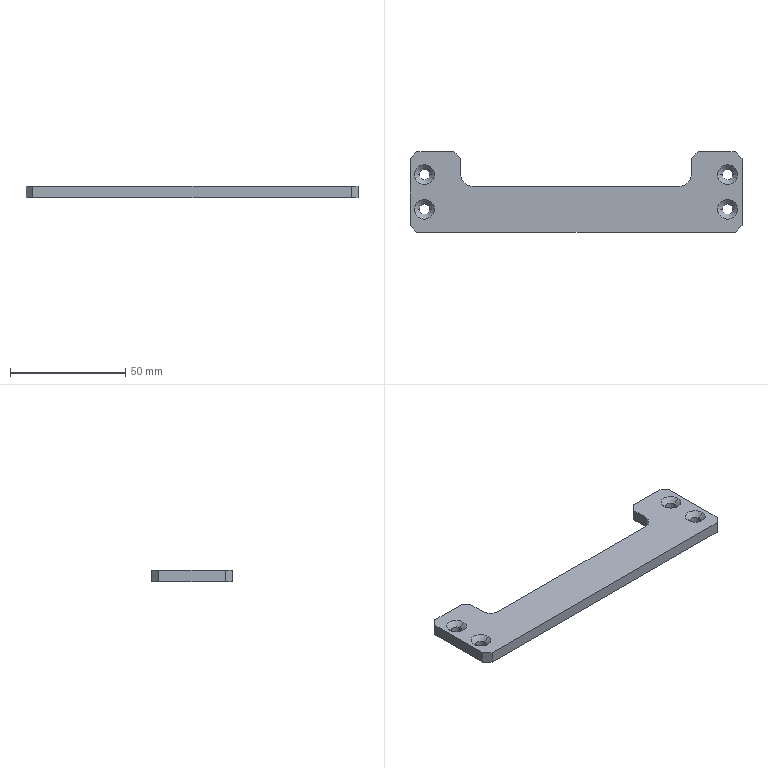Part | SolidWorks | features Chamfer 1, Extrusion 1, Fillet 1, HoleWzd 1, ICE 1 | 1 solid | 34 faces | box 144 x 35 x 5 mm | volume 17146 mm3 | plane 16 | cylinder 10 | cone 8 | commonest cylinder face diameters 4.5 x8 10 x2
STEP:
#1=CARTESIAN_POINT('',(-68.,7.5,2.95));
#2=VERTEX_POINT('',#1);
#3=CARTESIAN_POINT('',(-63.5,7.5,2.95));
#4=VERTEX_POINT('',#3);
#5=CARTESIAN_POINT('',(-65.75,7.5,2.95));
#6=DIRECTION('',(0.,0.,1.));
#7=DIRECTION('',(1.,0.,0.));
#8=AXIS2_PLACEMENT_3D('',#5,#6,#7);
#9=CIRCLE('',#8,2.25);
#10=EDGE_CURVE('',#2,#4,#9,.T.);
#11=ORIENTED_EDGE('',*,*,#10,.F.);
#12=CARTESIAN_POINT('',(-70.05,7.5,5.));
#13=VERTEX_POINT('',#12);
#14=CARTESIAN_POINT('',(-70.05,7.5,5.));
#15=DIRECTION('',(-0.7071,0.,0.7071));
#16=VECTOR('',#15,1000.);
#17=LINE('',#14,#16);
#18=EDGE_CURVE('',#2,#13,#17,.T.);
#19=ORIENTED_EDGE('',*,*,#18,.T.);
#20=CARTESIAN_POINT('',(-61.45,7.5,5.));
#21=VERTEX_POINT('',#20);
#22=CARTESIAN_POINT('',(-65.75,7.5,5.));
#23=DIRECTION('',(0.,0.,1.));
#24=DIRECTION('',(1.,0.,0.));
#25=AXIS2_PLACEMENT_3D('',#22,#23,#24);
#26=CIRCLE('',#25,4.3);
#27=EDGE_CURVE('',#13,#21,#26,.T.);
#28=ORIENTED_EDGE('',*,*,#27,.T.);
#29=CARTESIAN_POINT('',(-61.45,7.5,5.));
#30=DIRECTION('',(0.7071,0.,0.7071));
#31=VECTOR('',#30,1000.);
#32=LINE('',#29,#31);
#33=EDGE_CURVE('',#4,#21,#32,.T.);
#34=ORIENTED_EDGE('',*,*,#33,.F.);
#35=EDGE_LOOP('',(#11,#19,#28,#34));
#36=FACE_OUTER_BOUND('',#35,.T.);
#37=CARTESIAN_POINT('',(-65.75,7.5,5.));
#38=DIRECTION('',(0.,0.,1.));
#39=DIRECTION('',(1.,0.,0.));
#40=AXIS2_PLACEMENT_3D('',#37,#38,#39);
#41=CONICAL_SURFACE('',#40,4.3,0.7854);
#42=ADVANCED_FACE('',(#36),#41,.F.);
#43=CARTESIAN_POINT('',(-68.,7.5,0.));
#44=VERTEX_POINT('',#43);
#45=CARTESIAN_POINT('',(-63.5,7.5,0.));
#46=VERTEX_POINT('',#45);
#47=CARTESIAN_POINT('',(-65.75,7.5,0.));
#48=DIRECTION('',(0.,0.,1.));
#49=DIRECTION('',(1.,0.,0.));
#50=AXIS2_PLACEMENT_3D('',#47,#48,#49);
#51=CIRCLE('',#50,2.25);
#52=EDGE_CURVE('',#44,#46,#51,.T.);
#53=ORIENTED_EDGE('',*,*,#52,.F.);
#54=CARTESIAN_POINT('',(-68.,7.5,5.));
#55=DIRECTION('',(0.,0.,1.));
#56=VECTOR('',#55,1000.);
#57=LINE('',#54,#56);
#58=EDGE_CURVE('',#44,#2,#57,.T.);
#59=ORIENTED_EDGE('',*,*,#58,.T.);
#60=ORIENTED_EDGE('',*,*,#10,.T.);
#61=CARTESIAN_POINT('',(-63.5,7.5,5.));
#62=DIRECTION('',(0.,0.,1.));
#63=VECTOR('',#62,1000.);
#64=LINE('',#61,#63);
#65=EDGE_CURVE('',#46,#4,#64,.T.);
#66=ORIENTED_EDGE('',*,*,#65,.F.);
#67=EDGE_LOOP('',(#53,#59,#60,#66));
#68=FACE_OUTER_BOUND('',#67,.T.);
#69=CARTESIAN_POINT('',(-65.75,7.5,5.));
#70=DIRECTION('',(0.,0.,1.));
#71=DIRECTION('',(1.,0.,0.));
#72=AXIS2_PLACEMENT_3D('',#69,#70,#71);
#73=CYLINDRICAL_SURFACE('',#72,2.25);
#74=ADVANCED_FACE('',(#68),#73,.F.);
#75=CARTESIAN_POINT('',(-68.,-7.5,2.95));
#76=VERTEX_POINT('',#75);
#77=CARTESIAN_POINT('',(-63.5,-7.5,2.95));
#78=VERTEX_POINT('',#77);
#79=CARTESIAN_POINT('',(-65.75,-7.5,2.95));
#80=DIRECTION('',(0.,0.,1.));
#81=DIRECTION('',(1.,0.,0.));
#82=AXIS2_PLACEMENT_3D('',#79,#80,#81);
#83=CIRCLE('',#82,2.25);
#84=EDGE_CURVE('',#76,#78,#83,.T.);
#85=ORIENTED_EDGE('',*,*,#84,.F.);
#86=CARTESIAN_POINT('',(-70.05,-7.5,5.));
#87=VERTEX_POINT('',#86);
#88=CARTESIAN_POINT('',(-70.05,-7.5,5.));
#89=DIRECTION('',(-0.7071,0.,0.7071));
#90=VECTOR('',#89,1000.);
#91=LINE('',#88,#90);
#92=EDGE_CURVE('',#76,#87,#91,.T.);
#93=ORIENTED_EDGE('',*,*,#92,.T.);
#94=CARTESIAN_POINT('',(-61.45,-7.5,5.));
#95=VERTEX_POINT('',#94);
#96=CARTESIAN_POINT('',(-65.75,-7.5,5.));
#97=DIRECTION('',(0.,0.,1.));
#98=DIRECTION('',(1.,0.,0.));
#99=AXIS2_PLACEMENT_3D('',#96,#97,#98);
#100=CIRCLE('',#99,4.3);
#101=EDGE_CURVE('',#87,#95,#100,.T.);
#102=ORIENTED_EDGE('',*,*,#101,.T.);
#103=CARTESIAN_POINT('',(-61.45,-7.5,5.));
#104=DIRECTION('',(0.7071,0.,0.7071));
#105=VECTOR('',#104,1000.);
#106=LINE('',#103,#105);
#107=EDGE_CURVE('',#78,#95,#106,.T.);
#108=ORIENTED_EDGE('',*,*,#107,.F.);
#109=EDGE_LOOP('',(#85,#93,#102,#108));
#110=FACE_OUTER_BOUND('',#109,.T.);
#111=CARTESIAN_POINT('',(-65.75,-7.5,5.));
#112=DIRECTION('',(0.,0.,1.));
#113=DIRECTION('',(1.,0.,0.));
#114=AXIS2_PLACEMENT_3D('',#111,#112,#113);
#115=CONICAL_SURFACE('',#114,4.3,0.7854);
#116=ADVANCED_FACE('',(#110),#115,.F.);
#117=CARTESIAN_POINT('',(-68.,-7.5,0.));
#118=VERTEX_POINT('',#117);
#119=CARTESIAN_POINT('',(-63.5,-7.5,0.));
#120=VERTEX_POINT('',#119);
#121=CARTESIAN_POINT('',(-65.75,-7.5,0.));
#122=DIRECTION('',(0.,0.,1.));
#123=DIRECTION('',(1.,0.,0.));
#124=AXIS2_PLACEMENT_3D('',#121,#122,#123);
#125=CIRCLE('',#124,2.25);
#126=EDGE_CURVE('',#118,#120,#125,.T.);
#127=ORIENTED_EDGE('',*,*,#126,.F.);
#128=CARTESIAN_POINT('',(-68.,-7.5,5.));
#129=DIRECTION('',(0.,0.,1.));
#130=VECTOR('',#129,1000.);
#131=LINE('',#128,#130);
#132=EDGE_CURVE('',#118,#76,#131,.T.);
#133=ORIENTED_EDGE('',*,*,#132,.T.);
#134=ORIENTED_EDGE('',*,*,#84,.T.);
#135=CARTESIAN_POINT('',(-63.5,-7.5,5.));
#136=DIRECTION('',(0.,0.,1.));
#137=VECTOR('',#136,1000.);
#138=LINE('',#135,#137);
#139=EDGE_CURVE('',#120,#78,#138,.T.);
#140=ORIENTED_EDGE('',*,*,#139,.F.);
#141=EDGE_LOOP('',(#127,#133,#134,#140));
#142=FACE_OUTER_BOUND('',#141,.T.);
#143=CARTESIAN_POINT('',(-65.75,-7.5,5.));
#144=DIRECTION('',(0.,0.,1.));
#145=DIRECTION('',(1.,0.,0.));
#146=AXIS2_PLACEMENT_3D('',#143,#144,#145);
#147=CYLINDRICAL_SURFACE('',#146,2.25);
#148=ADVANCED_FACE('',(#142),#147,.F.);
#149=CARTESIAN_POINT('',(63.5,7.5,2.95));
#150=VERTEX_POINT('',#149);
#151=CARTESIAN_POINT('',(68.,7.5,2.95));
#152=VERTEX_POINT('',#151);
#153=CARTESIAN_POINT('',(65.75,7.5,2.95));
#154=DIRECTION('',(0.,0.,1.));
#155=DIRECTION('',(1.,0.,0.));
#156=AXIS2_PLACEMENT_3D('',#153,#154,#155);
#157=CIRCLE('',#156,2.25);
#158=EDGE_CURVE('',#150,#152,#157,.T.);
#159=ORIENTED_EDGE('',*,*,#158,.F.);
#160=CARTESIAN_POINT('',(61.45,7.5,5.));
#161=VERTEX_POINT('',#160);
#162=CARTESIAN_POINT('',(61.45,7.5,5.));
#163=DIRECTION('',(-0.7071,0.,0.7071));
#164=VECTOR('',#163,1000.);
#165=LINE('',#162,#164);
#166=EDGE_CURVE('',#150,#161,#165,.T.);
#167=ORIENTED_EDGE('',*,*,#166,.T.);
#168=CARTESIAN_POINT('',(70.05,7.5,5.));
#169=VERTEX_POINT('',#168);
#170=CARTESIAN_POINT('',(65.75,7.5,5.));
#171=DIRECTION('',(0.,0.,1.));
#172=DIRECTION('',(1.,0.,0.));
#173=AXIS2_PLACEMENT_3D('',#170,#171,#172);
#174=CIRCLE('',#173,4.3);
#175=EDGE_CURVE('',#161,#169,#174,.T.);
#176=ORIENTED_EDGE('',*,*,#175,.T.);
#177=CARTESIAN_POINT('',(70.05,7.5,5.));
#178=DIRECTION('',(0.7071,0.,0.7071));
#179=VECTOR('',#178,1000.);
#180=LINE('',#177,#179);
#181=EDGE_CURVE('',#152,#169,#180,.T.);
#182=ORIENTED_EDGE('',*,*,#181,.F.);
#183=EDGE_LOOP('',(#159,#167,#176,#182));
#184=FACE_OUTER_BOUND('',#183,.T.);
#185=CARTESIAN_POINT('',(65.75,7.5,5.));
#186=DIRECTION('',(0.,0.,1.));
#187=DIRECTION('',(1.,0.,0.));
#188=AXIS2_PLACEMENT_3D('',#185,#186,#187);
#189=CONICAL_SURFACE('',#188,4.3,0.7854);
#190=ADVANCED_FACE('',(#184),#189,.F.);
#191=CARTESIAN_POINT('',(63.5,7.5,0.));
#192=VERTEX_POINT('',#191);
#193=CARTESIAN_POINT('',(68.,7.5,0.));
#194=VERTEX_POINT('',#193);
#195=CARTESIAN_POINT('',(65.75,7.5,0.));
#196=DIRECTION('',(0.,0.,1.));
#197=DIRECTION('',(1.,0.,0.));
#198=AXIS2_PLACEMENT_3D('',#195,#196,#197);
#199=CIRCLE('',#198,2.25);
#200=EDGE_CURVE('',#192,#194,#199,.T.);
#201=ORIENTED_EDGE('',*,*,#200,.F.);
#202=CARTESIAN_POINT('',(63.5,7.5,5.));
#203=DIRECTION('',(0.,0.,1.));
#204=VECTOR('',#203,1000.);
#205=LINE('',#202,#204);
#206=EDGE_CURVE('',#192,#150,#205,.T.);
#207=ORIENTED_EDGE('',*,*,#206,.T.);
#208=ORIENTED_EDGE('',*,*,#158,.T.);
#209=CARTESIAN_POINT('',(68.,7.5,5.));
#210=DIRECTION('',(0.,0.,1.));
#211=VECTOR('',#210,1000.);
#212=LINE('',#209,#211);
#213=EDGE_CURVE('',#194,#152,#212,.T.);
#214=ORIENTED_EDGE('',*,*,#213,.F.);
#215=EDGE_LOOP('',(#201,#207,#208,#214));
#216=FACE_OUTER_BOUND('',#215,.T.);
#217=CARTESIAN_POINT('',(65.75,7.5,5.));
#218=DIRECTION('',(0.,0.,1.));
#219=DIRECTION('',(1.,0.,0.));
#220=AXIS2_PLACEMENT_3D('',#217,#218,#219);
#221=CYLINDRICAL_SURFACE('',#220,2.25);
#222=ADVANCED_FACE('',(#216),#221,.F.);
#223=CARTESIAN_POINT('',(63.5,-7.5,2.95));
#224=VERTEX_POINT('',#223);
#225=CARTESIAN_POINT('',(68.,-7.5,2.95));
#226=VERTEX_POINT('',#225);
#227=CARTESIAN_POINT('',(65.75,-7.5,2.95));
#228=DIRECTION('',(0.,0.,1.));
#229=DIRECTION('',(1.,0.,0.));
#230=AXIS2_PLACEMENT_3D('',#227,#228,#229);
#231=CIRCLE('',#230,2.25);
#232=EDGE_CURVE('',#224,#226,#231,.T.);
#233=ORIENTED_EDGE('',*,*,#232,.F.);
#234=CARTESIAN_POINT('',(61.45,-7.5,5.));
#235=VERTEX_POINT('',#234);
#236=CARTESIAN_POINT('',(61.45,-7.5,5.));
#237=DIRECTION('',(-0.7071,0.,0.7071));
#238=VECTOR('',#237,1000.);
#239=LINE('',#236,#238);
#240=EDGE_CURVE('',#224,#235,#239,.T.);
#241=ORIENTED_EDGE('',*,*,#240,.T.);
#242=CARTESIAN_POINT('',(70.05,-7.5,5.));
#243=VERTEX_POINT('',#242);
#244=CARTESIAN_POINT('',(65.75,-7.5,5.));
#245=DIRECTION('',(0.,0.,1.));
#246=DIRECTION('',(1.,0.,0.));
#247=AXIS2_PLACEMENT_3D('',#244,#245,#246);
#248=CIRCLE('',#247,4.3);
#249=EDGE_CURVE('',#235,#243,#248,.T.);
#250=ORIENTED_EDGE('',*,*,#249,.T.);
#251=CARTESIAN_POINT('',(70.05,-7.5,5.));
#252=DIRECTION('',(0.7071,0.,0.7071));
#253=VECTOR('',#252,1000.);
#254=LINE('',#251,#253);
#255=EDGE_CURVE('',#226,#243,#254,.T.);
#256=ORIENTED_EDGE('',*,*,#255,.F.);
#257=EDGE_LOOP('',(#233,#241,#250,#256));
#258=FACE_OUTER_BOUND('',#257,.T.);
#259=CARTESIAN_POINT('',(65.75,-7.5,5.));
#260=DIRECTION('',(0.,0.,1.));
#261=DIRECTION('',(1.,0.,0.));
#262=AXIS2_PLACEMENT_3D('',#259,#260,#261);
#263=CONICAL_SURFACE('',#262,4.3,0.7854);
#264=ADVANCED_FACE('',(#258),#263,.F.);
#265=CARTESIAN_POINT('',(63.5,-7.5,0.));
#266=VERTEX_POINT('',#265);
#267=CARTESIAN_POINT('',(68.,-7.5,0.));
#268=VERTEX_POINT('',#267);
#269=CARTESIAN_POINT('',(65.75,-7.5,0.));
#270=DIRECTION('',(0.,0.,1.));
#271=DIRECTION('',(1.,0.,0.));
#272=AXIS2_PLACEMENT_3D('',#269,#270,#271);
#273=CIRCLE('',#272,2.25);
#274=EDGE_CURVE('',#266,#268,#273,.T.);
#275=ORIENTED_EDGE('',*,*,#274,.F.);
#276=CARTESIAN_POINT('',(63.5,-7.5,5.));
#277=DIRECTION('',(0.,0.,1.));
#278=VECTOR('',#277,1000.);
#279=LINE('',#276,#278);
#280=EDGE_CURVE('',#266,#224,#279,.T.);
#281=ORIENTED_EDGE('',*,*,#280,.T.);
#282=ORIENTED_EDGE('',*,*,#232,.T.);
#283=CARTESIAN_POINT('',(68.,-7.5,5.));
#284=DIRECTION('',(0.,0.,1.));
#285=VECTOR('',#284,1000.);
#286=LINE('',#283,#285);
#287=EDGE_CURVE('',#268,#226,#286,.T.);
#288=ORIENTED_EDGE('',*,*,#287,.F.);
#289=EDGE_LOOP('',(#275,#281,#282,#288));
#290=FACE_OUTER_BOUND('',#289,.T.);
#291=CARTESIAN_POINT('',(65.75,-7.5,5.));
#292=DIRECTION('',(0.,0.,1.));
#293=DIRECTION('',(1.,0.,0.));
#294=AXIS2_PLACEMENT_3D('',#291,#292,#293);
#295=CYLINDRICAL_SURFACE('',#294,2.25);
#296=ADVANCED_FACE('',(#290),#295,.F.);
#297=CARTESIAN_POINT('',(-53.,17.5,5.));
#298=VERTEX_POINT('',#297);
#299=CARTESIAN_POINT('',(-69.,17.5,5.));
#300=VERTEX_POINT('',#299);
#301=CARTESIAN_POINT('',(-72.,17.5,5.));
#302=DIRECTION('',(-1.,0.,0.));
#303=VECTOR('',#302,1000.);
#304=LINE('',#301,#303);
#305=EDGE_CURVE('',#298,#300,#304,.T.);
#306=ORIENTED_EDGE('',*,*,#305,.F.);
#307=CARTESIAN_POINT('',(-53.,17.5,0.));
#308=VERTEX_POINT('',#307);
#309=CARTESIAN_POINT('',(-53.,17.5,5.));
#310=DIRECTION('',(0.,0.,-1.));
#311=VECTOR('',#310,1000.);
#312=LINE('',#309,#311);
#313=EDGE_CURVE('',#298,#308,#312,.T.);
#314=ORIENTED_EDGE('',*,*,#313,.T.);
#315=CARTESIAN_POINT('',(-69.,17.5,0.));
#316=VERTEX_POINT('',#315);
#317=CARTESIAN_POINT('',(-72.,17.5,0.));
#318=DIRECTION('',(-1.,0.,0.));
#319=VECTOR('',#318,1000.);
#320=LINE('',#317,#319);
#321=EDGE_CURVE('',#308,#316,#320,.T.);
#322=ORIENTED_EDGE('',*,*,#321,.T.);
#323=CARTESIAN_POINT('',(-69.,17.5,5.));
#324=DIRECTION('',(0.,0.,1.));
#325=VECTOR('',#324,1000.);
#326=LINE('',#323,#325);
#327=EDGE_CURVE('',#316,#300,#326,.T.);
#328=ORIENTED_EDGE('',*,*,#327,.T.);
#329=EDGE_LOOP('',(#306,#314,#322,#328));
#330=FACE_OUTER_BOUND('',#329,.T.);
#331=CARTESIAN_POINT('',(-72.,17.5,5.));
#332=DIRECTION('',(0.,-1.,0.));
#333=DIRECTION('',(0.,0.,-1.));
#334=AXIS2_PLACEMENT_3D('',#331,#332,#333);
#335=PLANE('',#334);
#336=ADVANCED_FACE('',(#330),#335,.F.);
#337=CARTESIAN_POINT('',(72.,-14.5,0.));
#338=VERTEX_POINT('',#337);
#339=CARTESIAN_POINT('',(72.,14.5,0.));
#340=VERTEX_POINT('',#339);
#341=CARTESIAN_POINT('',(72.,-17.5,0.));
#342=DIRECTION('',(0.,1.,0.));
#343=VECTOR('',#342,1000.);
#344=LINE('',#341,#343);
#345=EDGE_CURVE('',#338,#340,#344,.T.);
#346=ORIENTED_EDGE('',*,*,#345,.T.);
#347=CARTESIAN_POINT('',(72.,14.5,5.));
#348=VERTEX_POINT('',#347);
#349=CARTESIAN_POINT('',(72.,14.5,5.));
#350=DIRECTION('',(0.,0.,1.));
#351=VECTOR('',#350,1000.);
#352=LINE('',#349,#351);
#353=EDGE_CURVE('',#340,#348,#352,.T.);
#354=ORIENTED_EDGE('',*,*,#353,.T.);
#355=CARTESIAN_POINT('',(72.,-14.5,5.));
#356=VERTEX_POINT('',#355);
#357=CARTESIAN_POINT('',(72.,-17.5,5.));
#358=DIRECTION('',(0.,1.,0.));
#359=VECTOR('',#358,1000.);
#360=LINE('',#357,#359);
#361=EDGE_CURVE('',#356,#348,#360,.T.);
#362=ORIENTED_EDGE('',*,*,#361,.F.);
#363=CARTESIAN_POINT('',(72.,-14.5,5.));
#364=DIRECTION('',(0.,0.,-1.));
#365=VECTOR('',#364,1000.);
#366=LINE('',#363,#365);
#367=EDGE_CURVE('',#356,#338,#366,.T.);
#368=ORIENTED_EDGE('',*,*,#367,.T.);
#369=EDGE_LOOP('',(#346,#354,#362,#368));
#370=FACE_OUTER_BOUND('',#369,.T.);
#371=CARTESIAN_POINT('',(72.,-17.5,5.));
#372=DIRECTION('',(-1.,0.,0.));
#373=DIRECTION('',(0.,0.,1.));
#374=AXIS2_PLACEMENT_3D('',#371,#372,#373);
#375=PLANE('',#374);
#376=ADVANCED_FACE('',(#370),#375,.F.);
#377=CARTESIAN_POINT('',(69.,17.5,0.));
#378=VERTEX_POINT('',#377);
#379=CARTESIAN_POINT('',(53.,17.5,0.));
#380=VERTEX_POINT('',#379);
#381=CARTESIAN_POINT('',(-72.,17.5,0.));
#382=DIRECTION('',(-1.,0.,0.));
#383=VECTOR('',#382,1000.);
#384=LINE('',#381,#383);
#385=EDGE_CURVE('',#378,#380,#384,.T.);
#386=ORIENTED_EDGE('',*,*,#385,.T.);
#387=CARTESIAN_POINT('',(53.,17.5,5.));
#388=VERTEX_POINT('',#387);
#389=CARTESIAN_POINT('',(53.,17.5,5.));
#390=DIRECTION('',(0.,0.,1.));
#391=VECTOR('',#390,1000.);
#392=LINE('',#389,#391);
#393=EDGE_CURVE('',#380,#388,#392,.T.);
#394=ORIENTED_EDGE('',*,*,#393,.T.);
#395=CARTESIAN_POINT('',(69.,17.5,5.));
#396=VERTEX_POINT('',#395);
#397=CARTESIAN_POINT('',(-72.,17.5,5.));
#398=DIRECTION('',(-1.,0.,0.));
#399=VECTOR('',#398,1000.);
#400=LINE('',#397,#399);
#401=EDGE_CURVE('',#396,#388,#400,.T.);
#402=ORIENTED_EDGE('',*,*,#401,.F.);
#403=CARTESIAN_POINT('',(69.,17.5,5.));
#404=DIRECTION('',(0.,0.,-1.));
#405=VECTOR('',#404,1000.);
#406=LINE('',#403,#405);
#407=EDGE_CURVE('',#396,#378,#406,.T.);
#408=ORIENTED_EDGE('',*,*,#407,.T.);
#409=EDGE_LOOP('',(#386,#394,#402,#408));
#410=FACE_OUTER_BOUND('',#409,.T.);
#411=CARTESIAN_POINT('',(-72.,17.5,5.));
#412=DIRECTION('',(0.,-1.,0.));
#413=DIRECTION('',(0.,0.,-1.));
#414=AXIS2_PLACEMENT_3D('',#411,#412,#413);
#415=PLANE('',#414);
#416=ADVANCED_FACE('',(#410),#415,.F.);
#417=CARTESIAN_POINT('',(-72.,14.5,0.));
#418=VERTEX_POINT('',#417);
#419=CARTESIAN_POINT('',(-72.,-14.5,0.));
#420=VERTEX_POINT('',#419);
#421=CARTESIAN_POINT('',(-72.,-17.5,0.));
#422=DIRECTION('',(0.,-1.,0.));
#423=VECTOR('',#422,1000.);
#424=LINE('',#421,#423);
#425=EDGE_CURVE('',#418,#420,#424,.T.);
#426=ORIENTED_EDGE('',*,*,#425,.T.);
#427=CARTESIAN_POINT('',(-72.,-14.5,5.));
#428=VERTEX_POINT('',#427);
#429=CARTESIAN_POINT('',(-72.,-14.5,5.));
#430=DIRECTION('',(0.,0.,1.));
#431=VECTOR('',#430,1000.);
#432=LINE('',#429,#431);
#433=EDGE_CURVE('',#420,#428,#432,.T.);
#434=ORIENTED_EDGE('',*,*,#433,.T.);
#435=CARTESIAN_POINT('',(-72.,14.5,5.));
#436=VERTEX_POINT('',#435);
#437=CARTESIAN_POINT('',(-72.,-17.5,5.));
#438=DIRECTION('',(0.,-1.,0.));
#439=VECTOR('',#438,1000.);
#440=LINE('',#437,#439);
#441=EDGE_CURVE('',#436,#428,#440,.T.);
#442=ORIENTED_EDGE('',*,*,#441,.F.);
#443=CARTESIAN_POINT('',(-72.,14.5,5.));
#444=DIRECTION('',(0.,0.,-1.));
#445=VECTOR('',#444,1000.);
#446=LINE('',#443,#445);
#447=EDGE_CURVE('',#436,#418,#446,.T.);
#448=ORIENTED_EDGE('',*,*,#447,.T.);
#449=EDGE_LOOP('',(#426,#434,#442,#448));
#450=FACE_OUTER_BOUND('',#449,.T.);
#451=CARTESIAN_POINT('',(-72.,-17.5,5.));
#452=DIRECTION('',(1.,0.,0.));
#453=DIRECTION('',(0.,0.,-1.));
#454=AXIS2_PLACEMENT_3D('',#451,#452,#453);
#455=PLANE('',#454);
#456=ADVANCED_FACE('',(#450),#455,.F.);
#457=CARTESIAN_POINT('',(-69.,-17.5,0.));
#458=VERTEX_POINT('',#457);
#459=CARTESIAN_POINT('',(69.,-17.5,0.));
#460=VERTEX_POINT('',#459);
#461=CARTESIAN_POINT('',(-72.,-17.5,0.));
#462=DIRECTION('',(1.,0.,0.));
#463=VECTOR('',#462,1000.);
#464=LINE('',#461,#463);
#465=EDGE_CURVE('',#458,#460,#464,.T.);
#466=ORIENTED_EDGE('',*,*,#465,.T.);
#467=CARTESIAN_POINT('',(69.,-17.5,5.));
#468=VERTEX_POINT('',#467);
#469=CARTESIAN_POINT('',(69.,-17.5,5.));
#470=DIRECTION('',(0.,0.,1.));
#471=VECTOR('',#470,1000.);
#472=LINE('',#469,#471);
#473=EDGE_CURVE('',#460,#468,#472,.T.);
#474=ORIENTED_EDGE('',*,*,#473,.T.);
#475=CARTESIAN_POINT('',(-69.,-17.5,5.));
#476=VERTEX_POINT('',#475);
#477=CARTESIAN_POINT('',(-72.,-17.5,5.));
#478=DIRECTION('',(1.,0.,0.));
#479=VECTOR('',#478,1000.);
#480=LINE('',#477,#479);
#481=EDGE_CURVE('',#476,#468,#480,.T.);
#482=ORIENTED_EDGE('',*,*,#481,.F.);
#483=CARTESIAN_POINT('',(-69.,-17.5,5.));
#484=DIRECTION('',(0.,0.,-1.));
#485=VECTOR('',#484,1000.);
#486=LINE('',#483,#485);
#487=EDGE_CURVE('',#476,#458,#486,.T.);
#488=ORIENTED_EDGE('',*,*,#487,.T.);
#489=EDGE_LOOP('',(#466,#474,#482,#488));
#490=FACE_OUTER_BOUND('',#489,.T.);
#491=CARTESIAN_POINT('',(-72.,-17.5,5.));
#492=DIRECTION('',(0.,1.,0.));
#493=DIRECTION('',(0.,0.,1.));
#494=AXIS2_PLACEMENT_3D('',#491,#492,#493);
#495=PLANE('',#494);
#496=ADVANCED_FACE('',(#490),#495,.F.);
#497=CARTESIAN_POINT('',(-65.75,7.5,5.));
#498=DIRECTION('',(0.,0.,1.));
#499=DIRECTION('',(1.,0.,0.));
#500=AXIS2_PLACEMENT_3D('',#497,#498,#499);
#501=CIRCLE('',#500,4.3);
#502=EDGE_CURVE('',#21,#13,#501,.T.);
#503=ORIENTED_EDGE('',*,*,#502,.F.);
#504=ORIENTED_EDGE('',*,*,#27,.F.);
#505=EDGE_LOOP('',(#503,#504));
#506=FACE_BOUND('',#505,.T.);
#507=CARTESIAN_POINT('',(-65.75,-7.5,5.));
#508=DIRECTION('',(0.,0.,1.));
#509=DIRECTION('',(1.,0.,0.));
#510=AXIS2_PLACEMENT_3D('',#507,#508,#509);
#511=CIRCLE('',#510,4.3);
#512=EDGE_CURVE('',#95,#87,#511,.T.);
#513=ORIENTED_EDGE('',*,*,#512,.F.);
#514=ORIENTED_EDGE('',*,*,#101,.F.);
#515=EDGE_LOOP('',(#513,#514));
#516=FACE_BOUND('',#515,.T.);
#517=CARTESIAN_POINT('',(65.75,7.5,5.));
#518=DIRECTION('',(0.,0.,1.));
#519=DIRECTION('',(1.,0.,0.));
#520=AXIS2_PLACEMENT_3D('',#517,#518,#519);
#521=CIRCLE('',#520,4.3);
#522=EDGE_CURVE('',#169,#161,#521,.T.);
#523=ORIENTED_EDGE('',*,*,#522,.F.);
#524=ORIENTED_EDGE('',*,*,#175,.F.);
#525=EDGE_LOOP('',(#523,#524));
#526=FACE_BOUND('',#525,.T.);
#527=CARTESIAN_POINT('',(65.75,-7.5,5.));
#528=DIRECTION('',(0.,0.,1.));
#529=DIRECTION('',(1.,0.,0.));
#530=AXIS2_PLACEMENT_3D('',#527,#528,#529);
#531=CIRCLE('',#530,4.3);
#532=EDGE_CURVE('',#243,#235,#531,.T.);
#533=ORIENTED_EDGE('',*,*,#532,.F.);
#534=ORIENTED_EDGE('',*,*,#249,.F.);
#535=EDGE_LOOP('',(#533,#534));
#536=FACE_BOUND('',#535,.T.);
#537=ORIENTED_EDGE('',*,*,#401,.T.);
#538=CARTESIAN_POINT('',(50.,14.5,5.));
#539=VERTEX_POINT('',#538);
#540=CARTESIAN_POINT('',(53.,17.5,5.));
#541=DIRECTION('',(-0.7071,-0.7071,0.));
#542=VECTOR('',#541,1000.);
#543=LINE('',#540,#542);
#544=EDGE_CURVE('',#388,#539,#543,.T.);
#545=ORIENTED_EDGE('',*,*,#544,.T.);
#546=CARTESIAN_POINT('',(50.,7.5,5.));
#547=VERTEX_POINT('',#546);
#548=CARTESIAN_POINT('',(50.,17.5,5.));
#549=DIRECTION('',(0.,1.,0.));
#550=VECTOR('',#549,1000.);
#551=LINE('',#548,#550);
#552=EDGE_CURVE('',#547,#539,#551,.T.);
#553=ORIENTED_EDGE('',*,*,#552,.F.);
#554=CARTESIAN_POINT('',(45.,2.5,5.));
#555=VERTEX_POINT('',#554);
#556=CARTESIAN_POINT('',(45.,7.5,5.));
#557=DIRECTION('',(0.,0.,-1.));
#558=DIRECTION('',(-1.,0.,0.));
#559=AXIS2_PLACEMENT_3D('',#556,#557,#558);
#560=CIRCLE('',#559,5.);
#561=EDGE_CURVE('',#547,#555,#560,.T.);
#562=ORIENTED_EDGE('',*,*,#561,.T.);
#563=CARTESIAN_POINT('',(-45.,2.5,5.));
#564=VERTEX_POINT('',#563);
#565=CARTESIAN_POINT('',(-50.,2.5,5.));
#566=DIRECTION('',(1.,0.,0.));
#567=VECTOR('',#566,1000.);
#568=LINE('',#565,#567);
#569=EDGE_CURVE('',#564,#555,#568,.T.);
#570=ORIENTED_EDGE('',*,*,#569,.F.);
#571=CARTESIAN_POINT('',(-50.,7.5,5.));
#572=VERTEX_POINT('',#571);
#573=CARTESIAN_POINT('',(-45.,7.5,5.));
#574=DIRECTION('',(0.,0.,-1.));
#575=DIRECTION('',(-1.,0.,0.));
#576=AXIS2_PLACEMENT_3D('',#573,#574,#575);
#577=CIRCLE('',#576,5.);
#578=EDGE_CURVE('',#564,#572,#577,.T.);
#579=ORIENTED_EDGE('',*,*,#578,.T.);
#580=CARTESIAN_POINT('',(-50.,14.5,5.));
#581=VERTEX_POINT('',#580);
#582=CARTESIAN_POINT('',(-50.,17.5,5.));
#583=DIRECTION('',(0.,-1.,0.));
#584=VECTOR('',#583,1000.);
#585=LINE('',#582,#584);
#586=EDGE_CURVE('',#581,#572,#585,.T.);
#587=ORIENTED_EDGE('',*,*,#586,.F.);
#588=CARTESIAN_POINT('',(-50.,14.5,5.));
#589=DIRECTION('',(-0.7071,0.7071,0.));
#590=VECTOR('',#589,1000.);
#591=LINE('',#588,#590);
#592=EDGE_CURVE('',#581,#298,#591,.T.);
#593=ORIENTED_EDGE('',*,*,#592,.T.);
#594=ORIENTED_EDGE('',*,*,#305,.T.);
#595=CARTESIAN_POINT('',(-72.,14.5,5.));
#596=DIRECTION('',(-0.7071,-0.7071,0.));
#597=VECTOR('',#596,1000.);
#598=LINE('',#595,#597);
#599=EDGE_CURVE('',#300,#436,#598,.T.);
#600=ORIENTED_EDGE('',*,*,#599,.T.);
#601=ORIENTED_EDGE('',*,*,#441,.T.);
#602=CARTESIAN_POINT('',(-69.,-17.5,5.));
#603=DIRECTION('',(0.7071,-0.7071,0.));
#604=VECTOR('',#603,1000.);
#605=LINE('',#602,#604);
#606=EDGE_CURVE('',#428,#476,#605,.T.);
#607=ORIENTED_EDGE('',*,*,#606,.T.);
#608=ORIENTED_EDGE('',*,*,#481,.T.);
#609=CARTESIAN_POINT('',(72.,-14.5,5.));
#610=DIRECTION('',(0.7071,0.7071,0.));
#611=VECTOR('',#610,1000.);
#612=LINE('',#609,#611);
#613=EDGE_CURVE('',#468,#356,#612,.T.);
#614=ORIENTED_EDGE('',*,*,#613,.T.);
#615=ORIENTED_EDGE('',*,*,#361,.T.);
#616=CARTESIAN_POINT('',(69.,17.5,5.));
#617=DIRECTION('',(-0.7071,0.7071,0.));
#618=VECTOR('',#617,1000.);
#619=LINE('',#616,#618);
#620=EDGE_CURVE('',#348,#396,#619,.T.);
#621=ORIENTED_EDGE('',*,*,#620,.T.);
#622=EDGE_LOOP('',(#537,#545,#553,#562,#570,#579,#587,#593,#594,#600,#601,#607,#608,#614,#615,#621));
#623=FACE_OUTER_BOUND('',#622,.T.);
#624=CARTESIAN_POINT('',(0.,0.,5.));
#625=DIRECTION('',(0.,0.,-1.));
#626=DIRECTION('',(-1.,0.,0.));
#627=AXIS2_PLACEMENT_3D('',#624,#625,#626);
#628=PLANE('',#627);
#629=ADVANCED_FACE('',(#506,#516,#526,#536,#623),#628,.F.);
#630=CARTESIAN_POINT('',(-45.,2.5,0.));
#631=VERTEX_POINT('',#630);
#632=CARTESIAN_POINT('',(45.,2.5,0.));
#633=VERTEX_POINT('',#632);
#634=CARTESIAN_POINT('',(-50.,2.5,0.));
#635=DIRECTION('',(1.,0.,0.));
#636=VECTOR('',#635,1000.);
#637=LINE('',#634,#636);
#638=EDGE_CURVE('',#631,#633,#637,.T.);
#639=ORIENTED_EDGE('',*,*,#638,.T.);
#640=CARTESIAN_POINT('',(50.,7.5,0.));
#641=VERTEX_POINT('',#640);
#642=CARTESIAN_POINT('',(45.,7.5,0.));
#643=DIRECTION('',(0.,0.,1.));
#644=DIRECTION('',(-1.,0.,0.));
#645=AXIS2_PLACEMENT_3D('',#642,#643,#644);
#646=CIRCLE('',#645,5.);
#647=EDGE_CURVE('',#633,#641,#646,.T.);
#648=ORIENTED_EDGE('',*,*,#647,.T.);
#649=CARTESIAN_POINT('',(50.,14.5,0.));
#650=VERTEX_POINT('',#649);
#651=CARTESIAN_POINT('',(50.,17.5,0.));
#652=DIRECTION('',(0.,1.,0.));
#653=VECTOR('',#652,1000.);
#654=LINE('',#651,#653);
#655=EDGE_CURVE('',#641,#650,#654,.T.);
#656=ORIENTED_EDGE('',*,*,#655,.T.);
#657=CARTESIAN_POINT('',(17.75,-17.75,0.));
#658=DIRECTION('',(0.7071,0.7071,0.));
#659=VECTOR('',#658,1000.);
#660=LINE('',#657,#659);
#661=EDGE_CURVE('',#650,#380,#660,.T.);
#662=ORIENTED_EDGE('',*,*,#661,.T.);
#663=ORIENTED_EDGE('',*,*,#385,.F.);
#664=CARTESIAN_POINT('',(43.25,43.25,0.));
#665=DIRECTION('',(0.7071,-0.7071,0.));
#666=VECTOR('',#665,1000.);
#667=LINE('',#664,#666);
#668=EDGE_CURVE('',#378,#340,#667,.T.);
#669=ORIENTED_EDGE('',*,*,#668,.T.);
#670=ORIENTED_EDGE('',*,*,#345,.F.);
#671=CARTESIAN_POINT('',(43.25,-43.25,0.));
#672=DIRECTION('',(-0.7071,-0.7071,0.));
#673=VECTOR('',#672,1000.);
#674=LINE('',#671,#673);
#675=EDGE_CURVE('',#338,#460,#674,.T.);
#676=ORIENTED_EDGE('',*,*,#675,.T.);
#677=ORIENTED_EDGE('',*,*,#465,.F.);
#678=CARTESIAN_POINT('',(-43.25,-43.25,0.));
#679=DIRECTION('',(-0.7071,0.7071,0.));
#680=VECTOR('',#679,1000.);
#681=LINE('',#678,#680);
#682=EDGE_CURVE('',#458,#420,#681,.T.);
#683=ORIENTED_EDGE('',*,*,#682,.T.);
#684=ORIENTED_EDGE('',*,*,#425,.F.);
#685=CARTESIAN_POINT('',(-43.25,43.25,0.));
#686=DIRECTION('',(0.7071,0.7071,0.));
#687=VECTOR('',#686,1000.);
#688=LINE('',#685,#687);
#689=EDGE_CURVE('',#418,#316,#688,.T.);
#690=ORIENTED_EDGE('',*,*,#689,.T.);
#691=ORIENTED_EDGE('',*,*,#321,.F.);
#692=CARTESIAN_POINT('',(-50.,14.5,0.));
#693=VERTEX_POINT('',#692);
#694=CARTESIAN_POINT('',(-17.75,-17.75,0.));
#695=DIRECTION('',(0.7071,-0.7071,0.));
#696=VECTOR('',#695,1000.);
#697=LINE('',#694,#696);
#698=EDGE_CURVE('',#308,#693,#697,.T.);
#699=ORIENTED_EDGE('',*,*,#698,.T.);
#700=CARTESIAN_POINT('',(-50.,7.5,0.));
#701=VERTEX_POINT('',#700);
#702=CARTESIAN_POINT('',(-50.,17.5,0.));
#703=DIRECTION('',(0.,-1.,0.));
#704=VECTOR('',#703,1000.);
#705=LINE('',#702,#704);
#706=EDGE_CURVE('',#693,#701,#705,.T.);
#707=ORIENTED_EDGE('',*,*,#706,.T.);
#708=CARTESIAN_POINT('',(-45.,7.5,0.));
#709=DIRECTION('',(0.,0.,1.));
#710=DIRECTION('',(-1.,0.,0.));
#711=AXIS2_PLACEMENT_3D('',#708,#709,#710);
#712=CIRCLE('',#711,5.);
#713=EDGE_CURVE('',#701,#631,#712,.T.);
#714=ORIENTED_EDGE('',*,*,#713,.T.);
#715=EDGE_LOOP('',(#639,#648,#656,#662,#663,#669,#670,#676,#677,#683,#684,#690,#691,#699,#707,#714));
#716=FACE_OUTER_BOUND('',#715,.T.);
#717=CARTESIAN_POINT('',(-65.75,7.5,0.));
#718=DIRECTION('',(0.,0.,1.));
#719=DIRECTION('',(1.,0.,0.));
#720=AXIS2_PLACEMENT_3D('',#717,#718,#719);
#721=CIRCLE('',#720,2.25);
#722=EDGE_CURVE('',#46,#44,#721,.T.);
#723=ORIENTED_EDGE('',*,*,#722,.T.);
#724=ORIENTED_EDGE('',*,*,#52,.T.);
#725=EDGE_LOOP('',(#723,#724));
#726=FACE_BOUND('',#725,.T.);
#727=CARTESIAN_POINT('',(-65.75,-7.5,0.));
#728=DIRECTION('',(0.,0.,1.));
#729=DIRECTION('',(1.,0.,0.));
#730=AXIS2_PLACEMENT_3D('',#727,#728,#729);
#731=CIRCLE('',#730,2.25);
#732=EDGE_CURVE('',#120,#118,#731,.T.);
#733=ORIENTED_EDGE('',*,*,#732,.T.);
#734=ORIENTED_EDGE('',*,*,#126,.T.);
#735=EDGE_LOOP('',(#733,#734));
#736=FACE_BOUND('',#735,.T.);
#737=CARTESIAN_POINT('',(65.75,7.5,0.));
#738=DIRECTION('',(0.,0.,1.));
#739=DIRECTION('',(1.,0.,0.));
#740=AXIS2_PLACEMENT_3D('',#737,#738,#739);
#741=CIRCLE('',#740,2.25);
#742=EDGE_CURVE('',#194,#192,#741,.T.);
#743=ORIENTED_EDGE('',*,*,#742,.T.);
#744=ORIENTED_EDGE('',*,*,#200,.T.);
#745=EDGE_LOOP('',(#743,#744));
#746=FACE_BOUND('',#745,.T.);
#747=CARTESIAN_POINT('',(65.75,-7.5,0.));
#748=DIRECTION('',(0.,0.,1.));
#749=DIRECTION('',(1.,0.,0.));
#750=AXIS2_PLACEMENT_3D('',#747,#748,#749);
#751=CIRCLE('',#750,2.25);
#752=EDGE_CURVE('',#268,#266,#751,.T.);
#753=ORIENTED_EDGE('',*,*,#752,.T.);
#754=ORIENTED_EDGE('',*,*,#274,.T.);
#755=EDGE_LOOP('',(#753,#754));
#756=FACE_BOUND('',#755,.T.);
#757=CARTESIAN_POINT('',(0.,0.,0.));
#758=DIRECTION('',(0.,0.,-1.));
#759=DIRECTION('',(-1.,0.,0.));
#760=AXIS2_PLACEMENT_3D('',#757,#758,#759);
#761=PLANE('',#760);
#762=ADVANCED_FACE('',(#716,#726,#736,#746,#756),#761,.T.);
#763=ORIENTED_EDGE('',*,*,#280,.F.);
#764=ORIENTED_EDGE('',*,*,#752,.F.);
#765=ORIENTED_EDGE('',*,*,#287,.T.);
#766=CARTESIAN_POINT('',(65.75,-7.5,2.95));
#767=DIRECTION('',(0.,0.,1.));
#768=DIRECTION('',(1.,0.,0.));
#769=AXIS2_PLACEMENT_3D('',#766,#767,#768);
#770=CIRCLE('',#769,2.25);
#771=EDGE_CURVE('',#226,#224,#770,.T.);
#772=ORIENTED_EDGE('',*,*,#771,.T.);
#773=EDGE_LOOP('',(#763,#764,#765,#772));
#774=FACE_OUTER_BOUND('',#773,.T.);
#775=CARTESIAN_POINT('',(65.75,-7.5,5.));
#776=DIRECTION('',(0.,0.,1.));
#777=DIRECTION('',(1.,0.,0.));
#778=AXIS2_PLACEMENT_3D('',#775,#776,#777);
#779=CYLINDRICAL_SURFACE('',#778,2.25);
#780=ADVANCED_FACE('',(#774),#779,.F.);
#781=ORIENTED_EDGE('',*,*,#240,.F.);
#782=ORIENTED_EDGE('',*,*,#771,.F.);
#783=ORIENTED_EDGE('',*,*,#255,.T.);
#784=ORIENTED_EDGE('',*,*,#532,.T.);
#785=EDGE_LOOP('',(#781,#782,#783,#784));
#786=FACE_OUTER_BOUND('',#785,.T.);
#787=CARTESIAN_POINT('',(65.75,-7.5,5.));
#788=DIRECTION('',(0.,0.,1.));
#789=DIRECTION('',(1.,0.,0.));
#790=AXIS2_PLACEMENT_3D('',#787,#788,#789);
#791=CONICAL_SURFACE('',#790,4.3,0.7854);
#792=ADVANCED_FACE('',(#786),#791,.F.);
#793=ORIENTED_EDGE('',*,*,#206,.F.);
#794=ORIENTED_EDGE('',*,*,#742,.F.);
#795=ORIENTED_EDGE('',*,*,#213,.T.);
#796=CARTESIAN_POINT('',(65.75,7.5,2.95));
#797=DIRECTION('',(0.,0.,1.));
#798=DIRECTION('',(1.,0.,0.));
#799=AXIS2_PLACEMENT_3D('',#796,#797,#798);
#800=CIRCLE('',#799,2.25);
#801=EDGE_CURVE('',#152,#150,#800,.T.);
#802=ORIENTED_EDGE('',*,*,#801,.T.);
#803=EDGE_LOOP('',(#793,#794,#795,#802));
#804=FACE_OUTER_BOUND('',#803,.T.);
#805=CARTESIAN_POINT('',(65.75,7.5,5.));
#806=DIRECTION('',(0.,0.,1.));
#807=DIRECTION('',(1.,0.,0.));
#808=AXIS2_PLACEMENT_3D('',#805,#806,#807);
#809=CYLINDRICAL_SURFACE('',#808,2.25);
#810=ADVANCED_FACE('',(#804),#809,.F.);
#811=ORIENTED_EDGE('',*,*,#166,.F.);
#812=ORIENTED_EDGE('',*,*,#801,.F.);
#813=ORIENTED_EDGE('',*,*,#181,.T.);
#814=ORIENTED_EDGE('',*,*,#522,.T.);
#815=EDGE_LOOP('',(#811,#812,#813,#814));
#816=FACE_OUTER_BOUND('',#815,.T.);
#817=CARTESIAN_POINT('',(65.75,7.5,5.));
#818=DIRECTION('',(0.,0.,1.));
#819=DIRECTION('',(1.,0.,0.));
#820=AXIS2_PLACEMENT_3D('',#817,#818,#819);
#821=CONICAL_SURFACE('',#820,4.3,0.7854);
#822=ADVANCED_FACE('',(#816),#821,.F.);
#823=ORIENTED_EDGE('',*,*,#132,.F.);
#824=ORIENTED_EDGE('',*,*,#732,.F.);
#825=ORIENTED_EDGE('',*,*,#139,.T.);
#826=CARTESIAN_POINT('',(-65.75,-7.5,2.95));
#827=DIRECTION('',(0.,0.,1.));
#828=DIRECTION('',(1.,0.,0.));
#829=AXIS2_PLACEMENT_3D('',#826,#827,#828);
#830=CIRCLE('',#829,2.25);
#831=EDGE_CURVE('',#78,#76,#830,.T.);
#832=ORIENTED_EDGE('',*,*,#831,.T.);
#833=EDGE_LOOP('',(#823,#824,#825,#832));
#834=FACE_OUTER_BOUND('',#833,.T.);
#835=CARTESIAN_POINT('',(-65.75,-7.5,5.));
#836=DIRECTION('',(0.,0.,1.));
#837=DIRECTION('',(1.,0.,0.));
#838=AXIS2_PLACEMENT_3D('',#835,#836,#837);
#839=CYLINDRICAL_SURFACE('',#838,2.25);
#840=ADVANCED_FACE('',(#834),#839,.F.);
#841=ORIENTED_EDGE('',*,*,#92,.F.);
#842=ORIENTED_EDGE('',*,*,#831,.F.);
#843=ORIENTED_EDGE('',*,*,#107,.T.);
#844=ORIENTED_EDGE('',*,*,#512,.T.);
#845=EDGE_LOOP('',(#841,#842,#843,#844));
#846=FACE_OUTER_BOUND('',#845,.T.);
#847=CARTESIAN_POINT('',(-65.75,-7.5,5.));
#848=DIRECTION('',(0.,0.,1.));
#849=DIRECTION('',(1.,0.,0.));
#850=AXIS2_PLACEMENT_3D('',#847,#848,#849);
#851=CONICAL_SURFACE('',#850,4.3,0.7854);
#852=ADVANCED_FACE('',(#846),#851,.F.);
#853=ORIENTED_EDGE('',*,*,#58,.F.);
#854=ORIENTED_EDGE('',*,*,#722,.F.);
#855=ORIENTED_EDGE('',*,*,#65,.T.);
#856=CARTESIAN_POINT('',(-65.75,7.5,2.95));
#857=DIRECTION('',(0.,0.,1.));
#858=DIRECTION('',(1.,0.,0.));
#859=AXIS2_PLACEMENT_3D('',#856,#857,#858);
#860=CIRCLE('',#859,2.25);
#861=EDGE_CURVE('',#4,#2,#860,.T.);
#862=ORIENTED_EDGE('',*,*,#861,.T.);
#863=EDGE_LOOP('',(#853,#854,#855,#862));
#864=FACE_OUTER_BOUND('',#863,.T.);
#865=CARTESIAN_POINT('',(-65.75,7.5,5.));
#866=DIRECTION('',(0.,0.,1.));
#867=DIRECTION('',(1.,0.,0.));
#868=AXIS2_PLACEMENT_3D('',#865,#866,#867);
#869=CYLINDRICAL_SURFACE('',#868,2.25);
#870=ADVANCED_FACE('',(#864),#869,.F.);
#871=ORIENTED_EDGE('',*,*,#18,.F.);
#872=ORIENTED_EDGE('',*,*,#861,.F.);
#873=ORIENTED_EDGE('',*,*,#33,.T.);
#874=ORIENTED_EDGE('',*,*,#502,.T.);
#875=EDGE_LOOP('',(#871,#872,#873,#874));
#876=FACE_OUTER_BOUND('',#875,.T.);
#877=CARTESIAN_POINT('',(-65.75,7.5,5.));
#878=DIRECTION('',(0.,0.,1.));
#879=DIRECTION('',(1.,0.,0.));
#880=AXIS2_PLACEMENT_3D('',#877,#878,#879);
#881=CONICAL_SURFACE('',#880,4.3,0.7854);
#882=ADVANCED_FACE('',(#876),#881,.F.);
#883=ORIENTED_EDGE('',*,*,#586,.T.);
#884=CARTESIAN_POINT('',(-50.,7.5,0.));
#885=DIRECTION('',(0.,0.,-1.));
#886=VECTOR('',#885,1000.);
#887=LINE('',#884,#886);
#888=EDGE_CURVE('',#572,#701,#887,.T.);
#889=ORIENTED_EDGE('',*,*,#888,.T.);
#890=ORIENTED_EDGE('',*,*,#706,.F.);
#891=CARTESIAN_POINT('',(-50.,14.5,0.));
#892=DIRECTION('',(0.,0.,1.));
#893=VECTOR('',#892,1000.);
#894=LINE('',#891,#893);
#895=EDGE_CURVE('',#693,#581,#894,.T.);
#896=ORIENTED_EDGE('',*,*,#895,.T.);
#897=EDGE_LOOP('',(#883,#889,#890,#896));
#898=FACE_OUTER_BOUND('',#897,.T.);
#899=CARTESIAN_POINT('',(-50.,17.5,0.));
#900=DIRECTION('',(-1.,0.,0.));
#901=DIRECTION('',(0.,0.,1.));
#902=AXIS2_PLACEMENT_3D('',#899,#900,#901);
#903=PLANE('',#902);
#904=ADVANCED_FACE('',(#898),#903,.F.);
#905=ORIENTED_EDGE('',*,*,#655,.F.);
#906=CARTESIAN_POINT('',(50.,7.5,5.));
#907=DIRECTION('',(0.,0.,1.));
#908=VECTOR('',#907,1000.);
#909=LINE('',#906,#908);
#910=EDGE_CURVE('',#641,#547,#909,.T.);
#911=ORIENTED_EDGE('',*,*,#910,.T.);
#912=ORIENTED_EDGE('',*,*,#552,.T.);
#913=CARTESIAN_POINT('',(50.,14.5,0.));
#914=DIRECTION('',(0.,0.,-1.));
#915=VECTOR('',#914,1000.);
#916=LINE('',#913,#915);
#917=EDGE_CURVE('',#539,#650,#916,.T.);
#918=ORIENTED_EDGE('',*,*,#917,.T.);
#919=EDGE_LOOP('',(#905,#911,#912,#918));
#920=FACE_OUTER_BOUND('',#919,.T.);
#921=CARTESIAN_POINT('',(50.,17.5,0.));
#922=DIRECTION('',(1.,0.,0.));
#923=DIRECTION('',(0.,0.,-1.));
#924=AXIS2_PLACEMENT_3D('',#921,#922,#923);
#925=PLANE('',#924);
#926=ADVANCED_FACE('',(#920),#925,.F.);
#927=ORIENTED_EDGE('',*,*,#569,.T.);
#928=CARTESIAN_POINT('',(45.,2.5,0.));
#929=DIRECTION('',(0.,0.,-1.));
#930=VECTOR('',#929,1000.);
#931=LINE('',#928,#930);
#932=EDGE_CURVE('',#555,#633,#931,.T.);
#933=ORIENTED_EDGE('',*,*,#932,.T.);
#934=ORIENTED_EDGE('',*,*,#638,.F.);
#935=CARTESIAN_POINT('',(-45.,2.5,5.));
#936=DIRECTION('',(0.,0.,1.));
#937=VECTOR('',#936,1000.);
#938=LINE('',#935,#937);
#939=EDGE_CURVE('',#631,#564,#938,.T.);
#940=ORIENTED_EDGE('',*,*,#939,.T.);
#941=EDGE_LOOP('',(#927,#933,#934,#940));
#942=FACE_OUTER_BOUND('',#941,.T.);
#943=CARTESIAN_POINT('',(-50.,2.5,0.));
#944=DIRECTION('',(0.,-1.,0.));
#945=DIRECTION('',(0.,0.,-1.));
#946=AXIS2_PLACEMENT_3D('',#943,#944,#945);
#947=PLANE('',#946);
#948=ADVANCED_FACE('',(#942),#947,.F.);
#949=ORIENTED_EDGE('',*,*,#661,.F.);
#950=ORIENTED_EDGE('',*,*,#917,.F.);
#951=ORIENTED_EDGE('',*,*,#544,.F.);
#952=ORIENTED_EDGE('',*,*,#393,.F.);
#953=EDGE_LOOP('',(#949,#950,#951,#952));
#954=FACE_OUTER_BOUND('',#953,.T.);
#955=CARTESIAN_POINT('',(53.,17.5,5.));
#956=DIRECTION('',(0.7071,-0.7071,0.));
#957=DIRECTION('',(0.,0.,1.));
#958=AXIS2_PLACEMENT_3D('',#955,#956,#957);
#959=PLANE('',#958);
#960=ADVANCED_FACE('',(#954),#959,.F.);
#961=ORIENTED_EDGE('',*,*,#698,.F.);
#962=ORIENTED_EDGE('',*,*,#313,.F.);
#963=ORIENTED_EDGE('',*,*,#592,.F.);
#964=ORIENTED_EDGE('',*,*,#895,.F.);
#965=EDGE_LOOP('',(#961,#962,#963,#964));
#966=FACE_OUTER_BOUND('',#965,.T.);
#967=CARTESIAN_POINT('',(-50.,14.5,0.));
#968=DIRECTION('',(-0.7071,-0.7071,0.));
#969=DIRECTION('',(0.,0.,1.));
#970=AXIS2_PLACEMENT_3D('',#967,#968,#969);
#971=PLANE('',#970);
#972=ADVANCED_FACE('',(#966),#971,.F.);
#973=ORIENTED_EDGE('',*,*,#620,.F.);
#974=ORIENTED_EDGE('',*,*,#353,.F.);
#975=ORIENTED_EDGE('',*,*,#668,.F.);
#976=ORIENTED_EDGE('',*,*,#407,.F.);
#977=EDGE_LOOP('',(#973,#974,#975,#976));
#978=FACE_OUTER_BOUND('',#977,.T.);
#979=CARTESIAN_POINT('',(69.,17.5,5.));
#980=DIRECTION('',(-0.7071,-0.7071,0.));
#981=DIRECTION('',(0.,0.,-1.));
#982=AXIS2_PLACEMENT_3D('',#979,#980,#981);
#983=PLANE('',#982);
#984=ADVANCED_FACE('',(#978),#983,.F.);
#985=ORIENTED_EDGE('',*,*,#613,.F.);
#986=ORIENTED_EDGE('',*,*,#473,.F.);
#987=ORIENTED_EDGE('',*,*,#675,.F.);
#988=ORIENTED_EDGE('',*,*,#367,.F.);
#989=EDGE_LOOP('',(#985,#986,#987,#988));
#990=FACE_OUTER_BOUND('',#989,.T.);
#991=CARTESIAN_POINT('',(72.,-14.5,5.));
#992=DIRECTION('',(-0.7071,0.7071,0.));
#993=DIRECTION('',(0.,0.,-1.));
#994=AXIS2_PLACEMENT_3D('',#991,#992,#993);
#995=PLANE('',#994);
#996=ADVANCED_FACE('',(#990),#995,.F.);
#997=ORIENTED_EDGE('',*,*,#606,.F.);
#998=ORIENTED_EDGE('',*,*,#433,.F.);
#999=ORIENTED_EDGE('',*,*,#682,.F.);
#1000=ORIENTED_EDGE('',*,*,#487,.F.);
#1001=EDGE_LOOP('',(#997,#998,#999,#1000));
#1002=FACE_OUTER_BOUND('',#1001,.T.);
#1003=CARTESIAN_POINT('',(-69.,-17.5,5.));
#1004=DIRECTION('',(0.7071,0.7071,0.));
#1005=DIRECTION('',(0.,0.,-1.));
#1006=AXIS2_PLACEMENT_3D('',#1003,#1004,#1005);
#1007=PLANE('',#1006);
#1008=ADVANCED_FACE('',(#1002),#1007,.F.);
#1009=ORIENTED_EDGE('',*,*,#599,.F.);
#1010=ORIENTED_EDGE('',*,*,#327,.F.);
#1011=ORIENTED_EDGE('',*,*,#689,.F.);
#1012=ORIENTED_EDGE('',*,*,#447,.F.);
#1013=EDGE_LOOP('',(#1009,#1010,#1011,#1012));
#1014=FACE_OUTER_BOUND('',#1013,.T.);
#1015=CARTESIAN_POINT('',(-72.,14.5,5.));
#1016=DIRECTION('',(0.7071,-0.7071,0.));
#1017=DIRECTION('',(0.,0.,-1.));
#1018=AXIS2_PLACEMENT_3D('',#1015,#1016,#1017);
#1019=PLANE('',#1018);
#1020=ADVANCED_FACE('',(#1014),#1019,.F.);
#1021=ORIENTED_EDGE('',*,*,#647,.F.);
#1022=ORIENTED_EDGE('',*,*,#932,.F.);
#1023=ORIENTED_EDGE('',*,*,#561,.F.);
#1024=ORIENTED_EDGE('',*,*,#910,.F.);
#1025=EDGE_LOOP('',(#1021,#1022,#1023,#1024));
#1026=FACE_OUTER_BOUND('',#1025,.T.);
#1027=CARTESIAN_POINT('',(45.,7.5,0.));
#1028=DIRECTION('',(0.,0.,-1.));
#1029=DIRECTION('',(-1.,0.,0.));
#1030=AXIS2_PLACEMENT_3D('',#1027,#1028,#1029);
#1031=CYLINDRICAL_SURFACE('',#1030,5.);
#1032=ADVANCED_FACE('',(#1026),#1031,.F.);
#1033=ORIENTED_EDGE('',*,*,#713,.F.);
#1034=ORIENTED_EDGE('',*,*,#888,.F.);
#1035=ORIENTED_EDGE('',*,*,#578,.F.);
#1036=ORIENTED_EDGE('',*,*,#939,.F.);
#1037=EDGE_LOOP('',(#1033,#1034,#1035,#1036));
#1038=FACE_OUTER_BOUND('',#1037,.T.);
#1039=CARTESIAN_POINT('',(-45.,7.5,0.));
#1040=DIRECTION('',(0.,0.,-1.));
#1041=DIRECTION('',(-1.,0.,0.));
#1042=AXIS2_PLACEMENT_3D('',#1039,#1040,#1041);
#1043=CYLINDRICAL_SURFACE('',#1042,5.);
#1044=ADVANCED_FACE('',(#1038),#1043,.F.);
#1045=CLOSED_SHELL('',(#42,#74,#116,#148,#190,#222,#264,#296,#336,#376,#416,#456,#496,#629,#762,#780,#792,#810,#822,#840,#852,#870,#882,#904,#926,#948,#960,#972,#984,#996,#1008,#1020,#1032,#1044));
#1046=MANIFOLD_SOLID_BREP('',#1045);
#1047=CARTESIAN_POINT('',(0.,0.,0.));
#1048=DIRECTION('',(0.,0.,1.));
#1049=DIRECTION('',(1.,0.,0.));
#1050=AXIS2_PLACEMENT_3D('',#1047,#1048,#1049);
#1051=(LENGTH_UNIT()NAMED_UNIT(*)SI_UNIT(.MILLI.,.METRE.));
#1052=UNCERTAINTY_MEASURE_WITH_UNIT(LENGTH_MEASURE(0.00001),#1051,'','');
#1053=(NAMED_UNIT(*)PLANE_ANGLE_UNIT()SI_UNIT($,.RADIAN.));
#1054=(NAMED_UNIT(*)SI_UNIT($,.STERADIAN.)SOLID_ANGLE_UNIT());
#1055=(GEOMETRIC_REPRESENTATION_CONTEXT(3)GLOBAL_UNCERTAINTY_ASSIGNED_CONTEXT((#1052))GLOBAL_UNIT_ASSIGNED_CONTEXT((#1051,#1053,#1054))REPRESENTATION_CONTEXT('',''));
#1056=ADVANCED_BREP_SHAPE_REPRESENTATION('',(#1046,#1050),#1055);